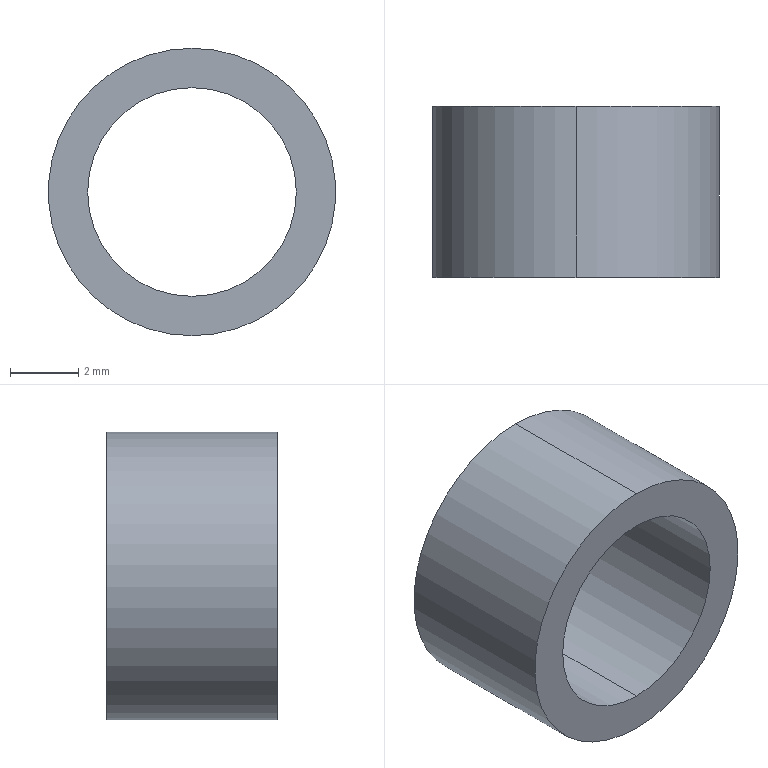Part | SolidWorks | features Revolution 1 | 1 solid | 6 faces | box 8.4 x 5 x 8.4 mm | volume 130.965 mm3 | cylinder 4 | plane 2 | commonest cylinder face diameters 6.1 x2 8.4 x2
STEP:
#1=CARTESIAN_POINT('',(0.,2.5,3.05));
#2=VERTEX_POINT('',#1);
#3=CARTESIAN_POINT('',(0.,2.5,-3.05));
#4=VERTEX_POINT('',#3);
#5=CARTESIAN_POINT('',(0.,2.5,0.));
#6=DIRECTION('',(0.,-1.,0.));
#7=DIRECTION('',(0.,0.,-1.));
#8=AXIS2_PLACEMENT_3D('',#5,#6,#7);
#9=CIRCLE('',#8,3.05);
#10=EDGE_CURVE('',#2,#4,#9,.T.);
#11=ORIENTED_EDGE('',*,*,#10,.F.);
#12=CARTESIAN_POINT('',(0.,-2.5,3.05));
#13=VERTEX_POINT('',#12);
#14=CARTESIAN_POINT('',(0.,0.,3.05));
#15=DIRECTION('',(0.,-1.,0.));
#16=VECTOR('',#15,1000.);
#17=LINE('',#14,#16);
#18=EDGE_CURVE('',#2,#13,#17,.T.);
#19=ORIENTED_EDGE('',*,*,#18,.T.);
#20=CARTESIAN_POINT('',(0.,-2.5,-3.05));
#21=VERTEX_POINT('',#20);
#22=CARTESIAN_POINT('',(0.,-2.5,0.));
#23=DIRECTION('',(0.,-1.,0.));
#24=DIRECTION('',(0.,0.,-1.));
#25=AXIS2_PLACEMENT_3D('',#22,#23,#24);
#26=CIRCLE('',#25,3.05);
#27=EDGE_CURVE('',#13,#21,#26,.T.);
#28=ORIENTED_EDGE('',*,*,#27,.T.);
#29=CARTESIAN_POINT('',(0.,0.,-3.05));
#30=DIRECTION('',(0.,-1.,0.));
#31=VECTOR('',#30,1000.);
#32=LINE('',#29,#31);
#33=EDGE_CURVE('',#4,#21,#32,.T.);
#34=ORIENTED_EDGE('',*,*,#33,.F.);
#35=EDGE_LOOP('',(#11,#19,#28,#34));
#36=FACE_OUTER_BOUND('',#35,.T.);
#37=CARTESIAN_POINT('',(0.,0.,0.));
#38=DIRECTION('',(0.,-1.,0.));
#39=DIRECTION('',(0.,0.,-1.));
#40=AXIS2_PLACEMENT_3D('',#37,#38,#39);
#41=CYLINDRICAL_SURFACE('',#40,3.05);
#42=ADVANCED_FACE('',(#36),#41,.F.);
#43=CARTESIAN_POINT('',(0.,2.5,-4.2));
#44=VERTEX_POINT('',#43);
#45=CARTESIAN_POINT('',(0.,2.5,4.2));
#46=VERTEX_POINT('',#45);
#47=CARTESIAN_POINT('',(0.,2.5,0.));
#48=DIRECTION('',(0.,-1.,0.));
#49=DIRECTION('',(0.,0.,-1.));
#50=AXIS2_PLACEMENT_3D('',#47,#48,#49);
#51=CIRCLE('',#50,4.2);
#52=EDGE_CURVE('',#44,#46,#51,.T.);
#53=ORIENTED_EDGE('',*,*,#52,.T.);
#54=CARTESIAN_POINT('',(0.,-2.5,4.2));
#55=VERTEX_POINT('',#54);
#56=CARTESIAN_POINT('',(0.,0.,4.2));
#57=DIRECTION('',(0.,-1.,0.));
#58=VECTOR('',#57,1000.);
#59=LINE('',#56,#58);
#60=EDGE_CURVE('',#46,#55,#59,.T.);
#61=ORIENTED_EDGE('',*,*,#60,.T.);
#62=CARTESIAN_POINT('',(0.,-2.5,-4.2));
#63=VERTEX_POINT('',#62);
#64=CARTESIAN_POINT('',(0.,-2.5,0.));
#65=DIRECTION('',(0.,-1.,0.));
#66=DIRECTION('',(0.,0.,-1.));
#67=AXIS2_PLACEMENT_3D('',#64,#65,#66);
#68=CIRCLE('',#67,4.2);
#69=EDGE_CURVE('',#63,#55,#68,.T.);
#70=ORIENTED_EDGE('',*,*,#69,.F.);
#71=CARTESIAN_POINT('',(0.,0.,-4.2));
#72=DIRECTION('',(0.,-1.,0.));
#73=VECTOR('',#72,1000.);
#74=LINE('',#71,#73);
#75=EDGE_CURVE('',#44,#63,#74,.T.);
#76=ORIENTED_EDGE('',*,*,#75,.F.);
#77=EDGE_LOOP('',(#53,#61,#70,#76));
#78=FACE_OUTER_BOUND('',#77,.T.);
#79=CARTESIAN_POINT('',(0.,0.,0.));
#80=DIRECTION('',(0.,-1.,0.));
#81=DIRECTION('',(0.,0.,-1.));
#82=AXIS2_PLACEMENT_3D('',#79,#80,#81);
#83=CYLINDRICAL_SURFACE('',#82,4.2);
#84=ADVANCED_FACE('',(#78),#83,.T.);
#85=ORIENTED_EDGE('',*,*,#60,.F.);
#86=CARTESIAN_POINT('',(0.,2.5,0.));
#87=DIRECTION('',(0.,-1.,0.));
#88=DIRECTION('',(0.,0.,-1.));
#89=AXIS2_PLACEMENT_3D('',#86,#87,#88);
#90=CIRCLE('',#89,4.2);
#91=EDGE_CURVE('',#46,#44,#90,.T.);
#92=ORIENTED_EDGE('',*,*,#91,.T.);
#93=ORIENTED_EDGE('',*,*,#75,.T.);
#94=CARTESIAN_POINT('',(0.,-2.5,0.));
#95=DIRECTION('',(0.,-1.,0.));
#96=DIRECTION('',(0.,0.,-1.));
#97=AXIS2_PLACEMENT_3D('',#94,#95,#96);
#98=CIRCLE('',#97,4.2);
#99=EDGE_CURVE('',#55,#63,#98,.T.);
#100=ORIENTED_EDGE('',*,*,#99,.F.);
#101=EDGE_LOOP('',(#85,#92,#93,#100));
#102=FACE_OUTER_BOUND('',#101,.T.);
#103=CARTESIAN_POINT('',(0.,0.,0.));
#104=DIRECTION('',(0.,-1.,0.));
#105=DIRECTION('',(0.,0.,-1.));
#106=AXIS2_PLACEMENT_3D('',#103,#104,#105);
#107=CYLINDRICAL_SURFACE('',#106,4.2);
#108=ADVANCED_FACE('',(#102),#107,.T.);
#109=CARTESIAN_POINT('',(0.,2.5,0.));
#110=DIRECTION('',(0.,-1.,0.));
#111=DIRECTION('',(0.,0.,-1.));
#112=AXIS2_PLACEMENT_3D('',#109,#110,#111);
#113=CIRCLE('',#112,3.05);
#114=EDGE_CURVE('',#4,#2,#113,.T.);
#115=ORIENTED_EDGE('',*,*,#114,.T.);
#116=ORIENTED_EDGE('',*,*,#10,.T.);
#117=EDGE_LOOP('',(#115,#116));
#118=FACE_BOUND('',#117,.T.);
#119=ORIENTED_EDGE('',*,*,#52,.F.);
#120=ORIENTED_EDGE('',*,*,#91,.F.);
#121=EDGE_LOOP('',(#119,#120));
#122=FACE_OUTER_BOUND('',#121,.T.);
#123=CARTESIAN_POINT('',(3.05,2.5,0.));
#124=DIRECTION('',(0.,1.,0.));
#125=DIRECTION('',(0.,0.,1.));
#126=AXIS2_PLACEMENT_3D('',#123,#124,#125);
#127=PLANE('',#126);
#128=ADVANCED_FACE('',(#118,#122),#127,.T.);
#129=ORIENTED_EDGE('',*,*,#18,.F.);
#130=ORIENTED_EDGE('',*,*,#114,.F.);
#131=ORIENTED_EDGE('',*,*,#33,.T.);
#132=CARTESIAN_POINT('',(0.,-2.5,0.));
#133=DIRECTION('',(0.,-1.,0.));
#134=DIRECTION('',(0.,0.,-1.));
#135=AXIS2_PLACEMENT_3D('',#132,#133,#134);
#136=CIRCLE('',#135,3.05);
#137=EDGE_CURVE('',#21,#13,#136,.T.);
#138=ORIENTED_EDGE('',*,*,#137,.T.);
#139=EDGE_LOOP('',(#129,#130,#131,#138));
#140=FACE_OUTER_BOUND('',#139,.T.);
#141=CARTESIAN_POINT('',(0.,0.,0.));
#142=DIRECTION('',(0.,-1.,0.));
#143=DIRECTION('',(0.,0.,-1.));
#144=AXIS2_PLACEMENT_3D('',#141,#142,#143);
#145=CYLINDRICAL_SURFACE('',#144,3.05);
#146=ADVANCED_FACE('',(#140),#145,.F.);
#147=ORIENTED_EDGE('',*,*,#69,.T.);
#148=ORIENTED_EDGE('',*,*,#99,.T.);
#149=EDGE_LOOP('',(#147,#148));
#150=FACE_OUTER_BOUND('',#149,.T.);
#151=ORIENTED_EDGE('',*,*,#137,.F.);
#152=ORIENTED_EDGE('',*,*,#27,.F.);
#153=EDGE_LOOP('',(#151,#152));
#154=FACE_BOUND('',#153,.T.);
#155=CARTESIAN_POINT('',(3.05,-2.5,0.));
#156=DIRECTION('',(0.,-1.,0.));
#157=DIRECTION('',(0.,0.,-1.));
#158=AXIS2_PLACEMENT_3D('',#155,#156,#157);
#159=PLANE('',#158);
#160=ADVANCED_FACE('',(#150,#154),#159,.T.);
#161=CLOSED_SHELL('',(#42,#84,#108,#128,#146,#160));
#162=MANIFOLD_SOLID_BREP('',#161);
#163=CARTESIAN_POINT('',(0.,0.,0.));
#164=DIRECTION('',(0.,0.,1.));
#165=DIRECTION('',(1.,0.,0.));
#166=AXIS2_PLACEMENT_3D('',#163,#164,#165);
#167=(LENGTH_UNIT()NAMED_UNIT(*)SI_UNIT(.MILLI.,.METRE.));
#168=UNCERTAINTY_MEASURE_WITH_UNIT(LENGTH_MEASURE(0.00001),#167,'','');
#169=(NAMED_UNIT(*)PLANE_ANGLE_UNIT()SI_UNIT($,.RADIAN.));
#170=(NAMED_UNIT(*)SI_UNIT($,.STERADIAN.)SOLID_ANGLE_UNIT());
#171=(GEOMETRIC_REPRESENTATION_CONTEXT(3)GLOBAL_UNCERTAINTY_ASSIGNED_CONTEXT((#168))GLOBAL_UNIT_ASSIGNED_CONTEXT((#167,#169,#170))REPRESENTATION_CONTEXT('',''));
#172=ADVANCED_BREP_SHAPE_REPRESENTATION('',(#162,#166),#171);